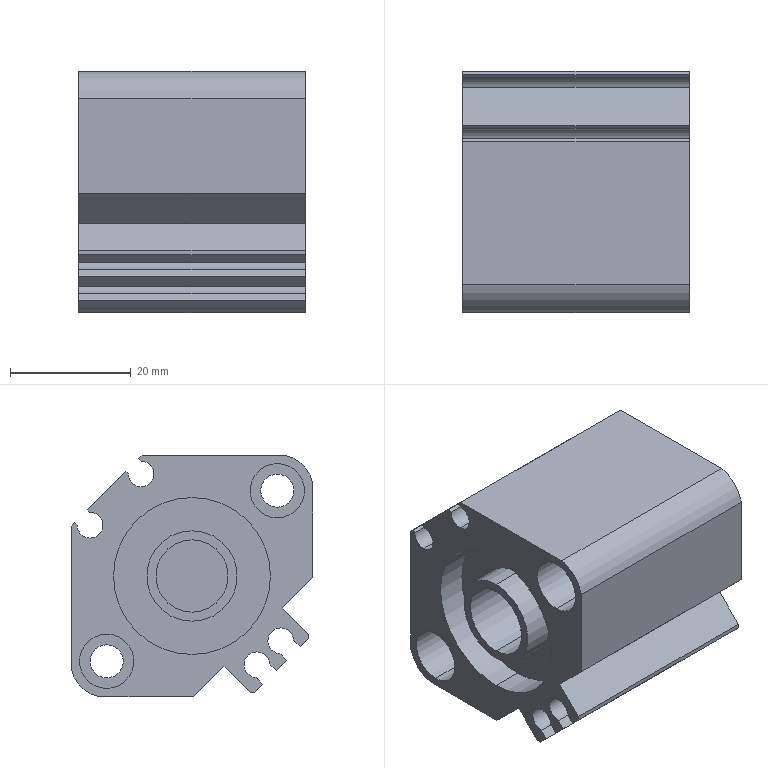Part | STEP file | 1_9 | 1 solid | 79 faces | box 37.5 x 40 x 40 mm | volume 38658 mm3 | cylinder 38 | plane 37 | cone 4 | commonest cylinder face diameters 4.26 x10 9 x8 4.134 x4 5.5 x4 12 x4 26 x4